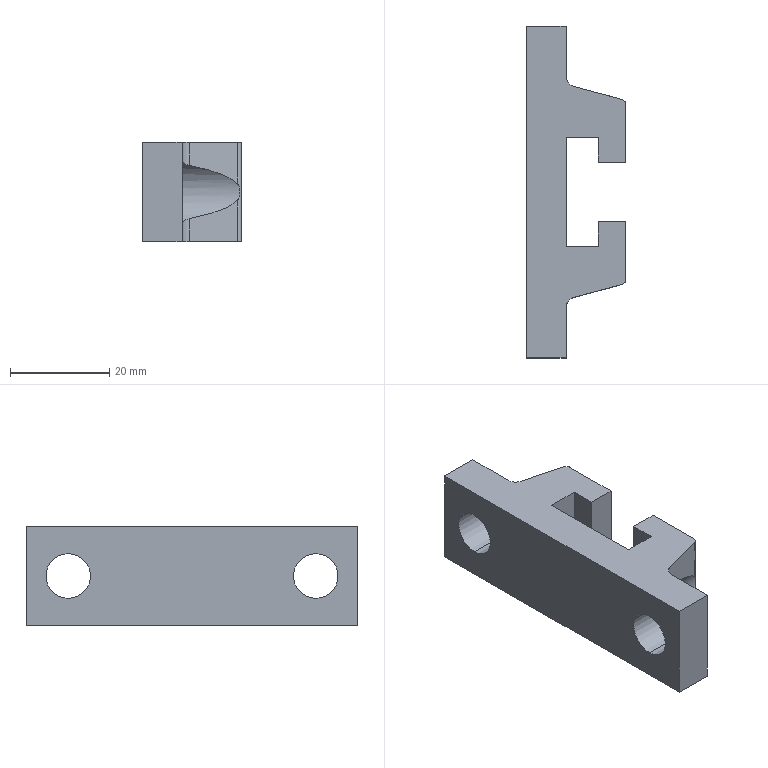Part | STEP file | _YA-05_CQ2.stp | 1 solid | 32 faces | box 20 x 67 x 20 mm | volume 14925 mm3 | plane 20 | cylinder 12 | commonest cylinder face diameters 4 x4 9 x4 2 x2 13 x2